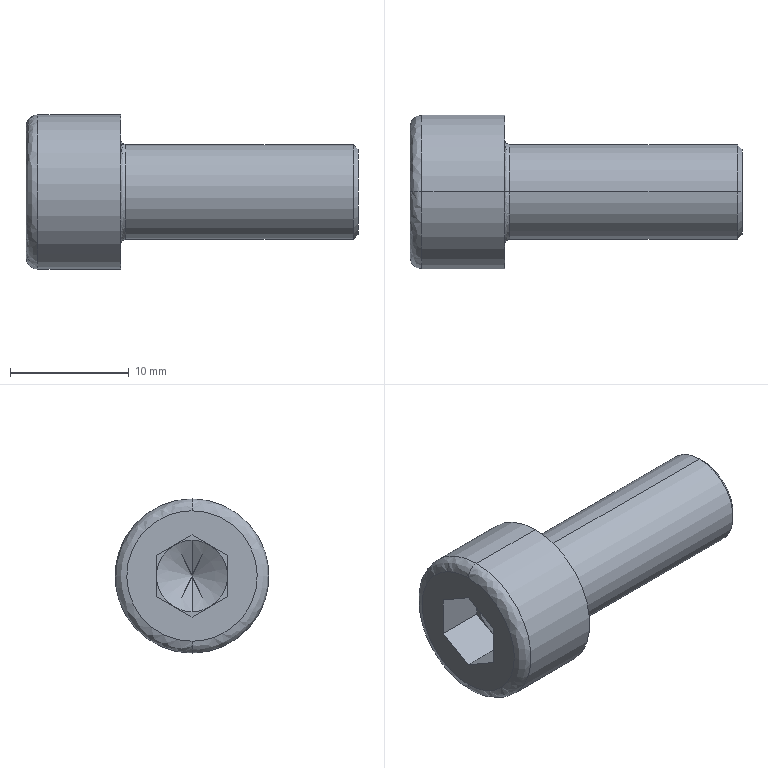Part | SolidWorks | features BaseBody 1 | 1 solid | 27 faces | box 28 x 13 x 13 mm | volume 1917 mm3 | plane 15 | spline 4 | cylinder 4 | cone 4 | commonest cylinder face diameters 8 x2 13 x2
STEP:
#1=CARTESIAN_POINT('',(8.,0.,4.4));
#2=VERTEX_POINT('',#1);
#3=CARTESIAN_POINT('',(8.,0.,-4.4));
#4=VERTEX_POINT('',#3);
#5=CARTESIAN_POINT('',(8.,0.,4.4));
#6=CARTESIAN_POINT('',(8.,0.2797,4.4));
#7=CARTESIAN_POINT('',(8.,0.6919,4.361));
#8=CARTESIAN_POINT('',(8.,1.16,4.249));
#9=CARTESIAN_POINT('',(8.,1.391,4.176));
#10=CARTESIAN_POINT('',(8.,1.489,4.141));
#11=CARTESIAN_POINT('',(8.,1.554,4.116));
#12=CARTESIAN_POINT('',(8.,1.585,4.105));
#13=CARTESIAN_POINT('',(8.,1.758,4.036));
#14=CARTESIAN_POINT('',(8.,1.96,3.944));
#15=CARTESIAN_POINT('',(8.,2.154,3.837));
#16=CARTESIAN_POINT('',(8.,2.282,3.763));
#17=CARTESIAN_POINT('',(8.,2.344,3.724));
#18=CARTESIAN_POINT('',(8.,2.662,3.517));
#19=CARTESIAN_POINT('',(8.,2.897,3.326));
#20=CARTESIAN_POINT('',(8.,3.219,3.004));
#21=CARTESIAN_POINT('',(8.,3.37,2.836));
#22=CARTESIAN_POINT('',(8.,3.509,2.656));
#23=CARTESIAN_POINT('',(8.,3.598,2.534));
#24=CARTESIAN_POINT('',(8.,3.642,2.47));
#25=CARTESIAN_POINT('',(8.,3.764,2.283));
#26=CARTESIAN_POINT('',(8.,3.876,2.092));
#27=CARTESIAN_POINT('',(8.,3.989,1.859));
#28=CARTESIAN_POINT('',(8.,4.042,1.74));
#29=CARTESIAN_POINT('',(8.,4.063,1.689));
#30=CARTESIAN_POINT('',(8.,4.077,1.654));
#31=CARTESIAN_POINT('',(8.,4.085,1.636));
#32=CARTESIAN_POINT('',(8.,4.297,1.1));
#33=CARTESIAN_POINT('',(8.,4.4,0.5592));
#34=CARTESIAN_POINT('',(8.,4.4,-0.2796));
#35=CARTESIAN_POINT('',(8.,4.361,-0.6917));
#36=CARTESIAN_POINT('',(8.,4.249,-1.16));
#37=CARTESIAN_POINT('',(8.,4.176,-1.391));
#38=CARTESIAN_POINT('',(8.,4.141,-1.489));
#39=CARTESIAN_POINT('',(8.,4.116,-1.554));
#40=CARTESIAN_POINT('',(8.,4.105,-1.585));
#41=CARTESIAN_POINT('',(8.,4.036,-1.758));
#42=CARTESIAN_POINT('',(8.,3.944,-1.96));
#43=CARTESIAN_POINT('',(8.,3.837,-2.154));
#44=CARTESIAN_POINT('',(8.,3.763,-2.282));
#45=CARTESIAN_POINT('',(8.,3.724,-2.344));
#46=CARTESIAN_POINT('',(8.,3.517,-2.662));
#47=CARTESIAN_POINT('',(8.,3.326,-2.897));
#48=CARTESIAN_POINT('',(8.,3.004,-3.219));
#49=CARTESIAN_POINT('',(8.,2.836,-3.37));
#50=CARTESIAN_POINT('',(8.,2.656,-3.509));
#51=CARTESIAN_POINT('',(8.,2.534,-3.598));
#52=CARTESIAN_POINT('',(8.,2.47,-3.642));
#53=CARTESIAN_POINT('',(8.,2.283,-3.764));
#54=CARTESIAN_POINT('',(8.,2.092,-3.876));
#55=CARTESIAN_POINT('',(8.,1.859,-3.989));
#56=CARTESIAN_POINT('',(8.,1.74,-4.042));
#57=CARTESIAN_POINT('',(8.,1.689,-4.063));
#58=CARTESIAN_POINT('',(8.,1.654,-4.077));
#59=CARTESIAN_POINT('',(8.,1.636,-4.085));
#60=CARTESIAN_POINT('',(8.,1.1,-4.297));
#61=CARTESIAN_POINT('',(8.,0.5597,-4.4));
#62=CARTESIAN_POINT('',(8.,0.,-4.4));
#63=B_SPLINE_CURVE_WITH_KNOTS('',3,(#5,#6,#7,#8,#9,#10,#11,#12,#13,#14,#15,#16,#17,#18,#19,#20,#21,#22,#23,#24,#25,#26,#27,#28,#29,#30,#31,#32,#33,#34,#35,#36,#37,#38,#39,#40,#41,#42,#43,#44,#45,#46,#47,#48,#49,#50,#51,#52,#53,#54,#55,#56,#57,#58,#59,#60,#61,#62),.UNSPECIFIED.,.F.,.F.,(4,1,1,1,2,2,1,2,2,2,1,2,2,1,1,1,2,2,2,1,1,1,2,2,1,2,2,2,1,2,2,1,1,1,2,2,4),(0.,0.0625,0.09375,0.1094,0.1172,0.125,0.1562,0.1719,0.1875,0.25,0.2812,0.2969,0.3125,0.3437,0.3594,0.3672,0.3711,0.375,0.5,0.5625,0.5937,0.6094,0.6172,0.625,0.6562,0.6719,0.6875,0.75,0.7812,0.7969,0.8125,0.8437,0.8594,0.8672,0.8711,0.875,1.),.UNSPECIFIED.);
#64=EDGE_CURVE('',#2,#4,#63,.T.);
#65=ORIENTED_EDGE('',*,*,#64,.F.);
#66=CARTESIAN_POINT('',(8.4,0.,4.));
#67=VERTEX_POINT('',#66);
#68=CARTESIAN_POINT('',(8.4,0.,4.4));
#69=DIRECTION('',(0.,-1.,0.));
#70=DIRECTION('',(0.,0.,1.));
#71=AXIS2_PLACEMENT_3D('',#68,#69,#70);
#72=CIRCLE('',#71,0.4);
#73=EDGE_CURVE('',#2,#67,#72,.T.);
#74=ORIENTED_EDGE('',*,*,#73,.T.);
#75=CARTESIAN_POINT('',(8.4,0.,-4.));
#76=VERTEX_POINT('',#75);
#77=CARTESIAN_POINT('',(8.4,0.,0.));
#78=DIRECTION('',(1.,0.,0.));
#79=DIRECTION('',(0.,0.,1.));
#80=AXIS2_PLACEMENT_3D('',#77,#78,#79);
#81=CIRCLE('',#80,4.);
#82=EDGE_CURVE('',#76,#67,#81,.T.);
#83=ORIENTED_EDGE('',*,*,#82,.F.);
#84=CARTESIAN_POINT('',(8.4,0.,-4.4));
#85=DIRECTION('',(0.,1.,0.));
#86=DIRECTION('',(0.,0.,-1.));
#87=AXIS2_PLACEMENT_3D('',#84,#85,#86);
#88=CIRCLE('',#87,0.4);
#89=EDGE_CURVE('',#4,#76,#88,.T.);
#90=ORIENTED_EDGE('',*,*,#89,.F.);
#91=EDGE_LOOP('',(#65,#74,#83,#90));
#92=FACE_OUTER_BOUND('',#91,.T.);
#93=CARTESIAN_POINT('',(8.,0.,-4.4));
#94=CARTESIAN_POINT('',(8.,8.8,-4.4));
#95=CARTESIAN_POINT('',(8.,8.8,4.4));
#96=CARTESIAN_POINT('',(8.,0.,4.4));
#97=CARTESIAN_POINT('',(8.,0.,-4.166));
#98=CARTESIAN_POINT('',(8.,8.331,-4.166));
#99=CARTESIAN_POINT('',(8.,8.331,4.166));
#100=CARTESIAN_POINT('',(8.,0.,4.166));
#101=CARTESIAN_POINT('',(8.166,0.,-4.));
#102=CARTESIAN_POINT('',(8.166,8.,-4.));
#103=CARTESIAN_POINT('',(8.166,8.,4.));
#104=CARTESIAN_POINT('',(8.166,0.,4.));
#105=CARTESIAN_POINT('',(8.4,0.,-4.));
#106=CARTESIAN_POINT('',(8.4,8.,-4.));
#107=CARTESIAN_POINT('',(8.4,8.,4.));
#108=CARTESIAN_POINT('',(8.4,0.,4.));
#109=(BOUNDED_SURFACE()B_SPLINE_SURFACE(3,3,((#93,#94,#95,#96),(#97,#98,#99,#100),(#101,#102,#103,#104),(#105,#106,#107,#108)),.UNSPECIFIED.,.F.,.F.,.T.)B_SPLINE_SURFACE_WITH_KNOTS((4,4),(4,4),(0.,1.),(0.,1.),.UNSPECIFIED.)GEOMETRIC_REPRESENTATION_ITEM()RATIONAL_B_SPLINE_SURFACE(((1.,0.3333,0.3333,1.),(0.8047,0.2682,0.2682,0.8047),(0.8047,0.2682,0.2682,0.8047),(1.,0.3333,0.3333,1.)))REPRESENTATION_ITEM('')SURFACE());
#110=ADVANCED_FACE('',(#92),#109,.F.);
#111=CARTESIAN_POINT('',(1.,0.,6.5));
#112=VERTEX_POINT('',#111);
#113=CARTESIAN_POINT('',(1.,0.,-6.5));
#114=VERTEX_POINT('',#113);
#115=CARTESIAN_POINT('',(1.,0.,0.));
#116=DIRECTION('',(1.,0.,0.));
#117=DIRECTION('',(0.,0.,1.));
#118=AXIS2_PLACEMENT_3D('',#115,#116,#117);
#119=CIRCLE('',#118,6.5);
#120=EDGE_CURVE('',#112,#114,#119,.T.);
#121=ORIENTED_EDGE('',*,*,#120,.F.);
#122=CARTESIAN_POINT('',(0.,0.,5.5));
#123=VERTEX_POINT('',#122);
#124=CARTESIAN_POINT('',(1.,0.,5.5));
#125=DIRECTION('',(0.,-1.,0.));
#126=DIRECTION('',(0.,0.,1.));
#127=AXIS2_PLACEMENT_3D('',#124,#125,#126);
#128=CIRCLE('',#127,1.);
#129=EDGE_CURVE('',#112,#123,#128,.T.);
#130=ORIENTED_EDGE('',*,*,#129,.T.);
#131=CARTESIAN_POINT('',(0.,0.,-5.5));
#132=VERTEX_POINT('',#131);
#133=CARTESIAN_POINT('',(0.,0.,5.5));
#134=CARTESIAN_POINT('',(0.,-11.,5.5));
#135=CARTESIAN_POINT('',(0.,-11.,-5.5));
#136=CARTESIAN_POINT('',(0.,0.,-5.5));
#137=(BOUNDED_CURVE()B_SPLINE_CURVE(3,(#133,#134,#135,#136),.UNSPECIFIED.,.F.,.F.)B_SPLINE_CURVE_WITH_KNOTS((4,4),(0.,1.),.UNSPECIFIED.)CURVE()GEOMETRIC_REPRESENTATION_ITEM()RATIONAL_B_SPLINE_CURVE((1.,0.3333,0.3333,1.))REPRESENTATION_ITEM(''));
#138=EDGE_CURVE('',#123,#132,#137,.T.);
#139=ORIENTED_EDGE('',*,*,#138,.T.);
#140=CARTESIAN_POINT('',(1.,0.,-5.5));
#141=DIRECTION('',(0.,1.,0.));
#142=DIRECTION('',(0.,0.,-1.));
#143=AXIS2_PLACEMENT_3D('',#140,#141,#142);
#144=CIRCLE('',#143,1.);
#145=EDGE_CURVE('',#114,#132,#144,.T.);
#146=ORIENTED_EDGE('',*,*,#145,.F.);
#147=EDGE_LOOP('',(#121,#130,#139,#146));
#148=FACE_OUTER_BOUND('',#147,.T.);
#149=CARTESIAN_POINT('',(1.,0.,6.5));
#150=CARTESIAN_POINT('',(1.,-13.,6.5));
#151=CARTESIAN_POINT('',(1.,-13.,-6.5));
#152=CARTESIAN_POINT('',(1.,0.,-6.5));
#153=CARTESIAN_POINT('',(0.4142,0.,6.5));
#154=CARTESIAN_POINT('',(0.4142,-13.,6.5));
#155=CARTESIAN_POINT('',(0.4142,-13.,-6.5));
#156=CARTESIAN_POINT('',(0.4142,0.,-6.5));
#157=CARTESIAN_POINT('',(0.,0.,6.086));
#158=CARTESIAN_POINT('',(0.,-12.172,6.086));
#159=CARTESIAN_POINT('',(0.,-12.172,-6.086));
#160=CARTESIAN_POINT('',(0.,0.,-6.086));
#161=CARTESIAN_POINT('',(0.,0.,5.5));
#162=CARTESIAN_POINT('',(0.,-11.,5.5));
#163=CARTESIAN_POINT('',(0.,-11.,-5.5));
#164=CARTESIAN_POINT('',(0.,0.,-5.5));
#165=(BOUNDED_SURFACE()B_SPLINE_SURFACE(3,3,((#149,#150,#151,#152),(#153,#154,#155,#156),(#157,#158,#159,#160),(#161,#162,#163,#164)),.UNSPECIFIED.,.F.,.F.,.F.)B_SPLINE_SURFACE_WITH_KNOTS((4,4),(4,4),(0.,1.),(0.,1.),.UNSPECIFIED.)GEOMETRIC_REPRESENTATION_ITEM()RATIONAL_B_SPLINE_SURFACE(((1.,0.3333,0.3333,1.),(0.8047,0.2682,0.2682,0.8047),(0.8047,0.2682,0.2682,0.8047),(1.,0.3333,0.3333,1.)))REPRESENTATION_ITEM('')SURFACE());
#166=ADVANCED_FACE('',(#148),#165,.T.);
#167=CARTESIAN_POINT('',(27.6,0.,4.));
#168=VERTEX_POINT('',#167);
#169=CARTESIAN_POINT('',(27.6,0.,-4.));
#170=VERTEX_POINT('',#169);
#171=CARTESIAN_POINT('',(27.6,0.,0.));
#172=DIRECTION('',(-1.,0.,0.));
#173=DIRECTION('',(0.,0.,1.));
#174=AXIS2_PLACEMENT_3D('',#171,#172,#173);
#175=CIRCLE('',#174,4.);
#176=EDGE_CURVE('',#168,#170,#175,.T.);
#177=ORIENTED_EDGE('',*,*,#176,.T.);
#178=CARTESIAN_POINT('',(28.,0.,-4.));
#179=DIRECTION('',(-1.,0.,0.));
#180=VECTOR('',#179,1000.);
#181=LINE('',#178,#180);
#182=EDGE_CURVE('',#170,#76,#181,.T.);
#183=ORIENTED_EDGE('',*,*,#182,.T.);
#184=ORIENTED_EDGE('',*,*,#82,.T.);
#185=CARTESIAN_POINT('',(28.,0.,4.));
#186=DIRECTION('',(-1.,0.,0.));
#187=VECTOR('',#186,1000.);
#188=LINE('',#185,#187);
#189=EDGE_CURVE('',#168,#67,#188,.T.);
#190=ORIENTED_EDGE('',*,*,#189,.F.);
#191=EDGE_LOOP('',(#177,#183,#184,#190));
#192=FACE_OUTER_BOUND('',#191,.T.);
#193=CARTESIAN_POINT('',(28.,0.,0.));
#194=DIRECTION('',(-1.,0.,0.));
#195=DIRECTION('',(0.,0.,1.));
#196=AXIS2_PLACEMENT_3D('',#193,#194,#195);
#197=CYLINDRICAL_SURFACE('',#196,4.);
#198=ADVANCED_FACE('',(#192),#197,.T.);
#199=CARTESIAN_POINT('',(28.,0.,3.6));
#200=VERTEX_POINT('',#199);
#201=CARTESIAN_POINT('',(28.,0.,-3.6));
#202=VERTEX_POINT('',#201);
#203=CARTESIAN_POINT('',(28.,0.,0.));
#204=DIRECTION('',(-1.,0.,0.));
#205=DIRECTION('',(0.,0.,1.));
#206=AXIS2_PLACEMENT_3D('',#203,#204,#205);
#207=CIRCLE('',#206,3.6);
#208=EDGE_CURVE('',#200,#202,#207,.T.);
#209=ORIENTED_EDGE('',*,*,#208,.T.);
#210=CARTESIAN_POINT('',(27.6,0.,-4.));
#211=DIRECTION('',(-0.7071,0.,-0.7071));
#212=VECTOR('',#211,1000.);
#213=LINE('',#210,#212);
#214=EDGE_CURVE('',#202,#170,#213,.T.);
#215=ORIENTED_EDGE('',*,*,#214,.T.);
#216=ORIENTED_EDGE('',*,*,#176,.F.);
#217=CARTESIAN_POINT('',(27.6,0.,4.));
#218=DIRECTION('',(-0.7071,0.,0.7071));
#219=VECTOR('',#218,1000.);
#220=LINE('',#217,#219);
#221=EDGE_CURVE('',#200,#168,#220,.T.);
#222=ORIENTED_EDGE('',*,*,#221,.F.);
#223=EDGE_LOOP('',(#209,#215,#216,#222));
#224=FACE_OUTER_BOUND('',#223,.T.);
#225=CARTESIAN_POINT('',(27.6,0.,0.));
#226=DIRECTION('',(-1.,0.,0.));
#227=DIRECTION('',(0.,0.,1.));
#228=AXIS2_PLACEMENT_3D('',#225,#226,#227);
#229=CONICAL_SURFACE('',#228,4.,0.7854);
#230=ADVANCED_FACE('',(#224),#229,.T.);
#231=CARTESIAN_POINT('',(8.,0.,-6.5));
#232=VERTEX_POINT('',#231);
#233=CARTESIAN_POINT('',(8.,0.,6.5));
#234=VERTEX_POINT('',#233);
#235=CARTESIAN_POINT('',(8.,0.,0.));
#236=DIRECTION('',(1.,0.,0.));
#237=DIRECTION('',(0.,0.,1.));
#238=AXIS2_PLACEMENT_3D('',#235,#236,#237);
#239=CIRCLE('',#238,6.5);
#240=EDGE_CURVE('',#232,#234,#239,.T.);
#241=ORIENTED_EDGE('',*,*,#240,.F.);
#242=CARTESIAN_POINT('',(8.,0.,-6.5));
#243=DIRECTION('',(-1.,0.,0.));
#244=VECTOR('',#243,1000.);
#245=LINE('',#242,#244);
#246=EDGE_CURVE('',#232,#114,#245,.T.);
#247=ORIENTED_EDGE('',*,*,#246,.T.);
#248=CARTESIAN_POINT('',(1.,0.,0.));
#249=DIRECTION('',(1.,0.,0.));
#250=DIRECTION('',(0.,0.,1.));
#251=AXIS2_PLACEMENT_3D('',#248,#249,#250);
#252=CIRCLE('',#251,6.5);
#253=EDGE_CURVE('',#114,#112,#252,.T.);
#254=ORIENTED_EDGE('',*,*,#253,.T.);
#255=CARTESIAN_POINT('',(8.,0.,6.5));
#256=DIRECTION('',(-1.,0.,0.));
#257=VECTOR('',#256,1000.);
#258=LINE('',#255,#257);
#259=EDGE_CURVE('',#234,#112,#258,.T.);
#260=ORIENTED_EDGE('',*,*,#259,.F.);
#261=EDGE_LOOP('',(#241,#247,#254,#260));
#262=FACE_OUTER_BOUND('',#261,.T.);
#263=CARTESIAN_POINT('',(8.,0.,0.));
#264=DIRECTION('',(-1.,0.,0.));
#265=DIRECTION('',(0.,0.,1.));
#266=AXIS2_PLACEMENT_3D('',#263,#264,#265);
#267=CYLINDRICAL_SURFACE('',#266,6.5);
#268=ADVANCED_FACE('',(#262),#267,.T.);
#269=CARTESIAN_POINT('',(5.732,0.,0.));
#270=VERTEX_POINT('',#269);
#271=CARTESIAN_POINT('',(4.,0.,3.));
#272=VERTEX_POINT('',#271);
#273=CARTESIAN_POINT('',(4.,0.,3.));
#274=DIRECTION('',(-0.5,0.,0.866));
#275=VECTOR('',#274,1000.);
#276=LINE('',#273,#275);
#277=EDGE_CURVE('',#270,#272,#276,.T.);
#278=ORIENTED_EDGE('',*,*,#277,.F.);
#279=CARTESIAN_POINT('',(4.,0.,-3.));
#280=VERTEX_POINT('',#279);
#281=CARTESIAN_POINT('',(4.,0.,-3.));
#282=DIRECTION('',(-0.5,0.,-0.866));
#283=VECTOR('',#282,1000.);
#284=LINE('',#281,#283);
#285=EDGE_CURVE('',#270,#280,#284,.T.);
#286=ORIENTED_EDGE('',*,*,#285,.T.);
#287=CARTESIAN_POINT('',(4.,-1.5,-2.598));
#288=VERTEX_POINT('',#287);
#289=CARTESIAN_POINT('',(4.,0.,0.));
#290=DIRECTION('',(1.,0.,0.));
#291=DIRECTION('',(0.,0.,1.));
#292=AXIS2_PLACEMENT_3D('',#289,#290,#291);
#293=CIRCLE('',#292,3.);
#294=EDGE_CURVE('',#288,#280,#293,.T.);
#295=ORIENTED_EDGE('',*,*,#294,.F.);
#296=CARTESIAN_POINT('',(4.,-3.,0.));
#297=VERTEX_POINT('',#296);
#298=CARTESIAN_POINT('',(4.,0.,0.));
#299=DIRECTION('',(-1.,0.,0.));
#300=DIRECTION('',(0.,0.,1.));
#301=AXIS2_PLACEMENT_3D('',#298,#299,#300);
#302=CIRCLE('',#301,3.);
#303=EDGE_CURVE('',#288,#297,#302,.T.);
#304=ORIENTED_EDGE('',*,*,#303,.T.);
#305=CARTESIAN_POINT('',(4.,-1.5,2.598));
#306=VERTEX_POINT('',#305);
#307=CARTESIAN_POINT('',(4.,0.,0.));
#308=DIRECTION('',(1.,0.,0.));
#309=DIRECTION('',(0.,0.,1.));
#310=AXIS2_PLACEMENT_3D('',#307,#308,#309);
#311=CIRCLE('',#310,3.);
#312=EDGE_CURVE('',#306,#297,#311,.T.);
#313=ORIENTED_EDGE('',*,*,#312,.F.);
#314=CARTESIAN_POINT('',(4.,0.,0.));
#315=DIRECTION('',(1.,0.,0.));
#316=DIRECTION('',(0.,0.,1.));
#317=AXIS2_PLACEMENT_3D('',#314,#315,#316);
#318=CIRCLE('',#317,3.);
#319=EDGE_CURVE('',#272,#306,#318,.T.);
#320=ORIENTED_EDGE('',*,*,#319,.F.);
#321=EDGE_LOOP('',(#278,#286,#295,#304,#313,#320));
#322=FACE_OUTER_BOUND('',#321,.T.);
#323=CARTESIAN_POINT('',(4.,0.,0.));
#324=DIRECTION('',(-1.,0.,0.));
#325=DIRECTION('',(0.,0.,1.));
#326=AXIS2_PLACEMENT_3D('',#323,#324,#325);
#327=CONICAL_SURFACE('',#326,3.,1.047);
#328=ADVANCED_FACE('',(#322),#327,.F.);
#329=ORIENTED_EDGE('',*,*,#182,.F.);
#330=CARTESIAN_POINT('',(27.6,0.,0.));
#331=DIRECTION('',(-1.,0.,0.));
#332=DIRECTION('',(0.,0.,1.));
#333=AXIS2_PLACEMENT_3D('',#330,#331,#332);
#334=CIRCLE('',#333,4.);
#335=EDGE_CURVE('',#170,#168,#334,.T.);
#336=ORIENTED_EDGE('',*,*,#335,.T.);
#337=ORIENTED_EDGE('',*,*,#189,.T.);
#338=CARTESIAN_POINT('',(8.4,0.,0.));
#339=DIRECTION('',(1.,0.,0.));
#340=DIRECTION('',(0.,0.,1.));
#341=AXIS2_PLACEMENT_3D('',#338,#339,#340);
#342=CIRCLE('',#341,4.);
#343=EDGE_CURVE('',#67,#76,#342,.T.);
#344=ORIENTED_EDGE('',*,*,#343,.T.);
#345=EDGE_LOOP('',(#329,#336,#337,#344));
#346=FACE_OUTER_BOUND('',#345,.T.);
#347=CARTESIAN_POINT('',(28.,0.,0.));
#348=DIRECTION('',(-1.,0.,0.));
#349=DIRECTION('',(0.,0.,1.));
#350=AXIS2_PLACEMENT_3D('',#347,#348,#349);
#351=CYLINDRICAL_SURFACE('',#350,4.);
#352=ADVANCED_FACE('',(#346),#351,.T.);
#353=ORIENTED_EDGE('',*,*,#73,.F.);
#354=CARTESIAN_POINT('',(8.,0.,-4.4));
#355=CARTESIAN_POINT('',(8.,-0.2797,-4.4));
#356=CARTESIAN_POINT('',(8.,-0.6919,-4.361));
#357=CARTESIAN_POINT('',(8.,-1.16,-4.249));
#358=CARTESIAN_POINT('',(8.,-1.391,-4.176));
#359=CARTESIAN_POINT('',(8.,-1.489,-4.141));
#360=CARTESIAN_POINT('',(8.,-1.554,-4.116));
#361=CARTESIAN_POINT('',(8.,-1.585,-4.105));
#362=CARTESIAN_POINT('',(8.,-1.758,-4.036));
#363=CARTESIAN_POINT('',(8.,-1.96,-3.944));
#364=CARTESIAN_POINT('',(8.,-2.154,-3.837));
#365=CARTESIAN_POINT('',(8.,-2.282,-3.763));
#366=CARTESIAN_POINT('',(8.,-2.344,-3.724));
#367=CARTESIAN_POINT('',(8.,-2.662,-3.517));
#368=CARTESIAN_POINT('',(8.,-2.897,-3.326));
#369=CARTESIAN_POINT('',(8.,-3.219,-3.004));
#370=CARTESIAN_POINT('',(8.,-3.37,-2.836));
#371=CARTESIAN_POINT('',(8.,-3.509,-2.656));
#372=CARTESIAN_POINT('',(8.,-3.598,-2.534));
#373=CARTESIAN_POINT('',(8.,-3.642,-2.47));
#374=CARTESIAN_POINT('',(8.,-3.764,-2.283));
#375=CARTESIAN_POINT('',(8.,-3.876,-2.092));
#376=CARTESIAN_POINT('',(8.,-3.989,-1.859));
#377=CARTESIAN_POINT('',(8.,-4.042,-1.74));
#378=CARTESIAN_POINT('',(8.,-4.063,-1.689));
#379=CARTESIAN_POINT('',(8.,-4.077,-1.654));
#380=CARTESIAN_POINT('',(8.,-4.085,-1.636));
#381=CARTESIAN_POINT('',(8.,-4.297,-1.1));
#382=CARTESIAN_POINT('',(8.,-4.4,-0.5592));
#383=CARTESIAN_POINT('',(8.,-4.4,0.2796));
#384=CARTESIAN_POINT('',(8.,-4.361,0.6917));
#385=CARTESIAN_POINT('',(8.,-4.249,1.16));
#386=CARTESIAN_POINT('',(8.,-4.176,1.391));
#387=CARTESIAN_POINT('',(8.,-4.141,1.489));
#388=CARTESIAN_POINT('',(8.,-4.116,1.554));
#389=CARTESIAN_POINT('',(8.,-4.105,1.585));
#390=CARTESIAN_POINT('',(8.,-4.036,1.758));
#391=CARTESIAN_POINT('',(8.,-3.944,1.96));
#392=CARTESIAN_POINT('',(8.,-3.837,2.154));
#393=CARTESIAN_POINT('',(8.,-3.763,2.282));
#394=CARTESIAN_POINT('',(8.,-3.724,2.344));
#395=CARTESIAN_POINT('',(8.,-3.517,2.662));
#396=CARTESIAN_POINT('',(8.,-3.326,2.897));
#397=CARTESIAN_POINT('',(8.,-3.004,3.219));
#398=CARTESIAN_POINT('',(8.,-2.836,3.37));
#399=CARTESIAN_POINT('',(8.,-2.656,3.509));
#400=CARTESIAN_POINT('',(8.,-2.534,3.598));
#401=CARTESIAN_POINT('',(8.,-2.47,3.642));
#402=CARTESIAN_POINT('',(8.,-2.283,3.764));
#403=CARTESIAN_POINT('',(8.,-2.092,3.876));
#404=CARTESIAN_POINT('',(8.,-1.859,3.989));
#405=CARTESIAN_POINT('',(8.,-1.74,4.042));
#406=CARTESIAN_POINT('',(8.,-1.689,4.063));
#407=CARTESIAN_POINT('',(8.,-1.654,4.077));
#408=CARTESIAN_POINT('',(8.,-1.636,4.085));
#409=CARTESIAN_POINT('',(8.,-1.1,4.297));
#410=CARTESIAN_POINT('',(8.,-0.5597,4.4));
#411=CARTESIAN_POINT('',(8.,0.,4.4));
#412=B_SPLINE_CURVE_WITH_KNOTS('',3,(#354,#355,#356,#357,#358,#359,#360,#361,#362,#363,#364,#365,#366,#367,#368,#369,#370,#371,#372,#373,#374,#375,#376,#377,#378,#379,#380,#381,#382,#383,#384,#385,#386,#387,#388,#389,#390,#391,#392,#393,#394,#395,#396,#397,#398,#399,#400,#401,#402,#403,#404,#405,#406,#407,#408,#409,#410,#411),.UNSPECIFIED.,.F.,.F.,(4,1,1,1,2,2,1,2,2,2,1,2,2,1,1,1,2,2,2,1,1,1,2,2,1,2,2,2,1,2,2,1,1,1,2,2,4),(0.,0.0625,0.09375,0.1094,0.1172,0.125,0.1563,0.1719,0.1875,0.25,0.2813,0.2969,0.3125,0.3438,0.3594,0.3672,0.3711,0.375,0.5,0.5625,0.5938,0.6094,0.6172,0.625,0.6563,0.6719,0.6875,0.75,0.7813,0.7969,0.8125,0.8438,0.8594,0.8672,0.8711,0.875,1.),.UNSPECIFIED.);
#413=EDGE_CURVE('',#4,#2,#412,.T.);
#414=ORIENTED_EDGE('',*,*,#413,.F.);
#415=ORIENTED_EDGE('',*,*,#89,.T.);
#416=ORIENTED_EDGE('',*,*,#343,.F.);
#417=EDGE_LOOP('',(#353,#414,#415,#416));
#418=FACE_OUTER_BOUND('',#417,.T.);
#419=CARTESIAN_POINT('',(8.,0.,4.4));
#420=CARTESIAN_POINT('',(8.,-8.8,4.4));
#421=CARTESIAN_POINT('',(8.,-8.8,-4.4));
#422=CARTESIAN_POINT('',(8.,0.,-4.4));
#423=CARTESIAN_POINT('',(8.,0.,4.166));
#424=CARTESIAN_POINT('',(8.,-8.331,4.166));
#425=CARTESIAN_POINT('',(8.,-8.331,-4.166));
#426=CARTESIAN_POINT('',(8.,0.,-4.166));
#427=CARTESIAN_POINT('',(8.166,0.,4.));
#428=CARTESIAN_POINT('',(8.166,-8.,4.));
#429=CARTESIAN_POINT('',(8.166,-8.,-4.));
#430=CARTESIAN_POINT('',(8.166,0.,-4.));
#431=CARTESIAN_POINT('',(8.4,0.,4.));
#432=CARTESIAN_POINT('',(8.4,-8.,4.));
#433=CARTESIAN_POINT('',(8.4,-8.,-4.));
#434=CARTESIAN_POINT('',(8.4,0.,-4.));
#435=(BOUNDED_SURFACE()B_SPLINE_SURFACE(3,3,((#419,#420,#421,#422),(#423,#424,#425,#426),(#427,#428,#429,#430),(#431,#432,#433,#434)),.UNSPECIFIED.,.F.,.F.,.T.)B_SPLINE_SURFACE_WITH_KNOTS((4,4),(4,4),(0.,1.),(0.,1.),.UNSPECIFIED.)GEOMETRIC_REPRESENTATION_ITEM()RATIONAL_B_SPLINE_SURFACE(((1.,0.3333,0.3333,1.),(0.8047,0.2682,0.2682,0.8047),(0.8047,0.2682,0.2682,0.8047),(1.,0.3333,0.3333,1.)))REPRESENTATION_ITEM('')SURFACE());
#436=ADVANCED_FACE('',(#418),#435,.F.);
#437=ORIENTED_EDGE('',*,*,#214,.F.);
#438=CARTESIAN_POINT('',(28.,0.,0.));
#439=DIRECTION('',(-1.,0.,0.));
#440=DIRECTION('',(0.,0.,1.));
#441=AXIS2_PLACEMENT_3D('',#438,#439,#440);
#442=CIRCLE('',#441,3.6);
#443=EDGE_CURVE('',#202,#200,#442,.T.);
#444=ORIENTED_EDGE('',*,*,#443,.T.);
#445=ORIENTED_EDGE('',*,*,#221,.T.);
#446=ORIENTED_EDGE('',*,*,#335,.F.);
#447=EDGE_LOOP('',(#437,#444,#445,#446));
#448=FACE_OUTER_BOUND('',#447,.T.);
#449=CARTESIAN_POINT('',(27.6,0.,0.));
#450=DIRECTION('',(-1.,0.,0.));
#451=DIRECTION('',(0.,0.,1.));
#452=AXIS2_PLACEMENT_3D('',#449,#450,#451);
#453=CONICAL_SURFACE('',#452,4.,0.7854);
#454=ADVANCED_FACE('',(#448),#453,.T.);
#455=CARTESIAN_POINT('',(8.,0.,0.));
#456=DIRECTION('',(1.,0.,0.));
#457=DIRECTION('',(0.,0.,1.));
#458=AXIS2_PLACEMENT_3D('',#455,#456,#457);
#459=CIRCLE('',#458,6.5);
#460=EDGE_CURVE('',#234,#232,#459,.T.);
#461=ORIENTED_EDGE('',*,*,#460,.T.);
#462=ORIENTED_EDGE('',*,*,#240,.T.);
#463=EDGE_LOOP('',(#461,#462));
#464=FACE_OUTER_BOUND('',#463,.T.);
#465=ORIENTED_EDGE('',*,*,#413,.T.);
#466=ORIENTED_EDGE('',*,*,#64,.T.);
#467=EDGE_LOOP('',(#465,#466));
#468=FACE_BOUND('',#467,.T.);
#469=CARTESIAN_POINT('',(8.,0.,0.));
#470=DIRECTION('',(1.,0.,0.));
#471=DIRECTION('',(0.,0.,-1.));
#472=AXIS2_PLACEMENT_3D('',#469,#470,#471);
#473=PLANE('',#472);
#474=ADVANCED_FACE('',(#464,#468),#473,.T.);
#475=ORIENTED_EDGE('',*,*,#208,.F.);
#476=ORIENTED_EDGE('',*,*,#443,.F.);
#477=EDGE_LOOP('',(#475,#476));
#478=FACE_OUTER_BOUND('',#477,.T.);
#479=CARTESIAN_POINT('',(28.,0.,0.));
#480=DIRECTION('',(1.,0.,0.));
#481=DIRECTION('',(0.,0.,-1.));
#482=AXIS2_PLACEMENT_3D('',#479,#480,#481);
#483=PLANE('',#482);
#484=ADVANCED_FACE('',(#478),#483,.T.);
#485=ORIENTED_EDGE('',*,*,#246,.F.);
#486=ORIENTED_EDGE('',*,*,#460,.F.);
#487=ORIENTED_EDGE('',*,*,#259,.T.);
#488=ORIENTED_EDGE('',*,*,#120,.T.);
#489=EDGE_LOOP('',(#485,#486,#487,#488));
#490=FACE_OUTER_BOUND('',#489,.T.);
#491=CARTESIAN_POINT('',(8.,0.,0.));
#492=DIRECTION('',(-1.,0.,0.));
#493=DIRECTION('',(0.,0.,1.));
#494=AXIS2_PLACEMENT_3D('',#491,#492,#493);
#495=CYLINDRICAL_SURFACE('',#494,6.5);
#496=ADVANCED_FACE('',(#490),#495,.T.);
#497=ORIENTED_EDGE('',*,*,#129,.F.);
#498=ORIENTED_EDGE('',*,*,#253,.F.);
#499=ORIENTED_EDGE('',*,*,#145,.T.);
#500=CARTESIAN_POINT('',(0.,0.,-5.5));
#501=CARTESIAN_POINT('',(0.,11.,-5.5));
#502=CARTESIAN_POINT('',(0.,11.,5.5));
#503=CARTESIAN_POINT('',(0.,0.,5.5));
#504=(BOUNDED_CURVE()B_SPLINE_CURVE(3,(#500,#501,#502,#503),.UNSPECIFIED.,.F.,.F.)B_SPLINE_CURVE_WITH_KNOTS((4,4),(0.,1.),.UNSPECIFIED.)CURVE()GEOMETRIC_REPRESENTATION_ITEM()RATIONAL_B_SPLINE_CURVE((1.,0.3333,0.3333,1.))REPRESENTATION_ITEM(''));
#505=EDGE_CURVE('',#132,#123,#504,.T.);
#506=ORIENTED_EDGE('',*,*,#505,.T.);
#507=EDGE_LOOP('',(#497,#498,#499,#506));
#508=FACE_OUTER_BOUND('',#507,.T.);
#509=CARTESIAN_POINT('',(1.,0.,-6.5));
#510=CARTESIAN_POINT('',(1.,13.,-6.5));
#511=CARTESIAN_POINT('',(1.,13.,6.5));
#512=CARTESIAN_POINT('',(1.,0.,6.5));
#513=CARTESIAN_POINT('',(0.4142,0.,-6.5));
#514=CARTESIAN_POINT('',(0.4142,13.,-6.5));
#515=CARTESIAN_POINT('',(0.4142,13.,6.5));
#516=CARTESIAN_POINT('',(0.4142,0.,6.5));
#517=CARTESIAN_POINT('',(0.,0.,-6.086));
#518=CARTESIAN_POINT('',(0.,12.172,-6.086));
#519=CARTESIAN_POINT('',(0.,12.172,6.086));
#520=CARTESIAN_POINT('',(0.,0.,6.086));
#521=CARTESIAN_POINT('',(0.,0.,-5.5));
#522=CARTESIAN_POINT('',(0.,11.,-5.5));
#523=CARTESIAN_POINT('',(0.,11.,5.5));
#524=CARTESIAN_POINT('',(0.,0.,5.5));
#525=(BOUNDED_SURFACE()B_SPLINE_SURFACE(3,3,((#509,#510,#511,#512),(#513,#514,#515,#516),(#517,#518,#519,#520),(#521,#522,#523,#524)),.UNSPECIFIED.,.F.,.F.,.F.)B_SPLINE_SURFACE_WITH_KNOTS((4,4),(4,4),(0.,1.),(0.,1.),.UNSPECIFIED.)GEOMETRIC_REPRESENTATION_ITEM()RATIONAL_B_SPLINE_SURFACE(((1.,0.3333,0.3333,1.),(0.8047,0.2682,0.2682,0.8047),(0.8047,0.2682,0.2682,0.8047),(1.,0.3333,0.3333,1.)))REPRESENTATION_ITEM('')SURFACE());
#526=ADVANCED_FACE('',(#508),#525,.T.);
#527=CARTESIAN_POINT('',(0.,3.,1.732));
#528=VERTEX_POINT('',#527);
#529=CARTESIAN_POINT('',(0.,3.,-1.732));
#530=VERTEX_POINT('',#529);
#531=CARTESIAN_POINT('',(0.,3.,0.));
#532=DIRECTION('',(0.,0.,-1.));
#533=VECTOR('',#532,1000.);
#534=LINE('',#531,#533);
#535=EDGE_CURVE('',#528,#530,#534,.T.);
#536=ORIENTED_EDGE('',*,*,#535,.F.);
#537=CARTESIAN_POINT('',(0.,0.,3.464));
#538=VERTEX_POINT('',#537);
#539=CARTESIAN_POINT('',(0.,0.,3.464));
#540=DIRECTION('',(0.,0.866,-0.5));
#541=VECTOR('',#540,1000.);
#542=LINE('',#539,#541);
#543=EDGE_CURVE('',#538,#528,#542,.T.);
#544=ORIENTED_EDGE('',*,*,#543,.F.);
#545=CARTESIAN_POINT('',(0.,-3.,1.732));
#546=VERTEX_POINT('',#545);
#547=CARTESIAN_POINT('',(0.,-3.,1.732));
#548=DIRECTION('',(0.,0.866,0.5));
#549=VECTOR('',#548,1000.);
#550=LINE('',#547,#549);
#551=EDGE_CURVE('',#546,#538,#550,.T.);
#552=ORIENTED_EDGE('',*,*,#551,.F.);
#553=CARTESIAN_POINT('',(0.,-3.,-1.732));
#554=VERTEX_POINT('',#553);
#555=CARTESIAN_POINT('',(0.,-3.,0.));
#556=DIRECTION('',(0.,0.,1.));
#557=VECTOR('',#556,1000.);
#558=LINE('',#555,#557);
#559=EDGE_CURVE('',#554,#546,#558,.T.);
#560=ORIENTED_EDGE('',*,*,#559,.F.);
#561=CARTESIAN_POINT('',(0.,0.,-3.464));
#562=VERTEX_POINT('',#561);
#563=CARTESIAN_POINT('',(0.,0.,-3.464));
#564=DIRECTION('',(0.,-0.866,0.5));
#565=VECTOR('',#564,1000.);
#566=LINE('',#563,#565);
#567=EDGE_CURVE('',#562,#554,#566,.T.);
#568=ORIENTED_EDGE('',*,*,#567,.F.);
#569=CARTESIAN_POINT('',(0.,3.,-1.732));
#570=DIRECTION('',(0.,-0.866,-0.5));
#571=VECTOR('',#570,1000.);
#572=LINE('',#569,#571);
#573=EDGE_CURVE('',#530,#562,#572,.T.);
#574=ORIENTED_EDGE('',*,*,#573,.F.);
#575=EDGE_LOOP('',(#536,#544,#552,#560,#568,#574));
#576=FACE_BOUND('',#575,.T.);
#577=ORIENTED_EDGE('',*,*,#505,.F.);
#578=ORIENTED_EDGE('',*,*,#138,.F.);
#579=EDGE_LOOP('',(#577,#578));
#580=FACE_OUTER_BOUND('',#579,.T.);
#581=CARTESIAN_POINT('',(0.,0.,0.));
#582=DIRECTION('',(1.,0.,0.));
#583=DIRECTION('',(0.,0.,-1.));
#584=AXIS2_PLACEMENT_3D('',#581,#582,#583);
#585=PLANE('',#584);
#586=ADVANCED_FACE('',(#576,#580),#585,.F.);
#587=CARTESIAN_POINT('',(4.,0.,-3.464));
#588=VERTEX_POINT('',#587);
#589=CARTESIAN_POINT('',(4.,0.,-3.464));
#590=DIRECTION('',(1.,0.,0.));
#591=VECTOR('',#590,1000.);
#592=LINE('',#589,#591);
#593=EDGE_CURVE('',#562,#588,#592,.T.);
#594=ORIENTED_EDGE('',*,*,#593,.T.);
#595=CARTESIAN_POINT('',(4.,1.5,-2.598));
#596=VERTEX_POINT('',#595);
#597=CARTESIAN_POINT('',(4.,0.,-3.464));
#598=DIRECTION('',(0.,0.866,0.5));
#599=VECTOR('',#598,1000.);
#600=LINE('',#597,#599);
#601=EDGE_CURVE('',#588,#596,#600,.T.);
#602=ORIENTED_EDGE('',*,*,#601,.T.);
#603=CARTESIAN_POINT('',(4.,3.,-1.732));
#604=VERTEX_POINT('',#603);
#605=CARTESIAN_POINT('',(4.,1.5,-2.598));
#606=DIRECTION('',(0.,0.866,0.5));
#607=VECTOR('',#606,1000.);
#608=LINE('',#605,#607);
#609=EDGE_CURVE('',#596,#604,#608,.T.);
#610=ORIENTED_EDGE('',*,*,#609,.T.);
#611=CARTESIAN_POINT('',(4.,3.,-1.732));
#612=DIRECTION('',(-1.,0.,0.));
#613=VECTOR('',#612,1000.);
#614=LINE('',#611,#613);
#615=EDGE_CURVE('',#604,#530,#614,.T.);
#616=ORIENTED_EDGE('',*,*,#615,.T.);
#617=ORIENTED_EDGE('',*,*,#573,.T.);
#618=EDGE_LOOP('',(#594,#602,#610,#616,#617));
#619=FACE_OUTER_BOUND('',#618,.T.);
#620=CARTESIAN_POINT('',(4.,0.,-3.464));
#621=DIRECTION('',(0.,-0.5,0.866));
#622=DIRECTION('',(0.,-0.866,-0.5));
#623=AXIS2_PLACEMENT_3D('',#620,#621,#622);
#624=PLANE('',#623);
#625=ADVANCED_FACE('',(#619),#624,.T.);
#626=ORIENTED_EDGE('',*,*,#615,.F.);
#627=CARTESIAN_POINT('',(4.,3.,0.));
#628=VERTEX_POINT('',#627);
#629=CARTESIAN_POINT('',(4.,3.,-3.464));
#630=DIRECTION('',(0.,0.,1.));
#631=VECTOR('',#630,1000.);
#632=LINE('',#629,#631);
#633=EDGE_CURVE('',#604,#628,#632,.T.);
#634=ORIENTED_EDGE('',*,*,#633,.T.);
#635=CARTESIAN_POINT('',(4.,3.,1.732));
#636=VERTEX_POINT('',#635);
#637=CARTESIAN_POINT('',(4.,3.,-3.464));
#638=DIRECTION('',(0.,0.,1.));
#639=VECTOR('',#638,1000.);
#640=LINE('',#637,#639);
#641=EDGE_CURVE('',#628,#636,#640,.T.);
#642=ORIENTED_EDGE('',*,*,#641,.T.);
#643=CARTESIAN_POINT('',(4.,3.,1.732));
#644=DIRECTION('',(-1.,0.,0.));
#645=VECTOR('',#644,1000.);
#646=LINE('',#643,#645);
#647=EDGE_CURVE('',#636,#528,#646,.T.);
#648=ORIENTED_EDGE('',*,*,#647,.T.);
#649=ORIENTED_EDGE('',*,*,#535,.T.);
#650=EDGE_LOOP('',(#626,#634,#642,#648,#649));
#651=FACE_OUTER_BOUND('',#650,.T.);
#652=CARTESIAN_POINT('',(4.,3.,-1.732));
#653=DIRECTION('',(0.,-1.,0.));
#654=DIRECTION('',(0.,0.,-1.));
#655=AXIS2_PLACEMENT_3D('',#652,#653,#654);
#656=PLANE('',#655);
#657=ADVANCED_FACE('',(#651),#656,.T.);
#658=ORIENTED_EDGE('',*,*,#647,.F.);
#659=CARTESIAN_POINT('',(4.,1.5,2.598));
#660=VERTEX_POINT('',#659);
#661=CARTESIAN_POINT('',(4.,3.,1.732));
#662=DIRECTION('',(0.,-0.866,0.5));
#663=VECTOR('',#662,1000.);
#664=LINE('',#661,#663);
#665=EDGE_CURVE('',#636,#660,#664,.T.);
#666=ORIENTED_EDGE('',*,*,#665,.T.);
#667=CARTESIAN_POINT('',(4.,0.,3.464));
#668=VERTEX_POINT('',#667);
#669=CARTESIAN_POINT('',(4.,3.,1.732));
#670=DIRECTION('',(0.,-0.866,0.5));
#671=VECTOR('',#670,1000.);
#672=LINE('',#669,#671);
#673=EDGE_CURVE('',#660,#668,#672,.T.);
#674=ORIENTED_EDGE('',*,*,#673,.T.);
#675=CARTESIAN_POINT('',(4.,0.,3.464));
#676=DIRECTION('',(-1.,0.,0.));
#677=VECTOR('',#676,1000.);
#678=LINE('',#675,#677);
#679=EDGE_CURVE('',#668,#538,#678,.T.);
#680=ORIENTED_EDGE('',*,*,#679,.T.);
#681=ORIENTED_EDGE('',*,*,#543,.T.);
#682=EDGE_LOOP('',(#658,#666,#674,#680,#681));
#683=FACE_OUTER_BOUND('',#682,.T.);
#684=CARTESIAN_POINT('',(4.,3.,1.732));
#685=DIRECTION('',(0.,-0.5,-0.866));
#686=DIRECTION('',(0.,0.866,-0.5));
#687=AXIS2_PLACEMENT_3D('',#684,#685,#686);
#688=PLANE('',#687);
#689=ADVANCED_FACE('',(#683),#688,.T.);
#690=ORIENTED_EDGE('',*,*,#679,.F.);
#691=CARTESIAN_POINT('',(4.,0.,3.464));
#692=DIRECTION('',(0.,-0.866,-0.5));
#693=VECTOR('',#692,1000.);
#694=LINE('',#691,#693);
#695=EDGE_CURVE('',#668,#306,#694,.T.);
#696=ORIENTED_EDGE('',*,*,#695,.T.);
#697=CARTESIAN_POINT('',(4.,-3.,1.732));
#698=VERTEX_POINT('',#697);
#699=CARTESIAN_POINT('',(4.,-1.5,2.598));
#700=DIRECTION('',(0.,-0.866,-0.5));
#701=VECTOR('',#700,1000.);
#702=LINE('',#699,#701);
#703=EDGE_CURVE('',#306,#698,#702,.T.);
#704=ORIENTED_EDGE('',*,*,#703,.T.);
#705=CARTESIAN_POINT('',(4.,-3.,1.732));
#706=DIRECTION('',(-1.,0.,0.));
#707=VECTOR('',#706,1000.);
#708=LINE('',#705,#707);
#709=EDGE_CURVE('',#698,#546,#708,.T.);
#710=ORIENTED_EDGE('',*,*,#709,.T.);
#711=ORIENTED_EDGE('',*,*,#551,.T.);
#712=EDGE_LOOP('',(#690,#696,#704,#710,#711));
#713=FACE_OUTER_BOUND('',#712,.T.);
#714=CARTESIAN_POINT('',(4.,0.,3.464));
#715=DIRECTION('',(0.,0.5,-0.866));
#716=DIRECTION('',(0.,0.866,0.5));
#717=AXIS2_PLACEMENT_3D('',#714,#715,#716);
#718=PLANE('',#717);
#719=ADVANCED_FACE('',(#713),#718,.T.);
#720=ORIENTED_EDGE('',*,*,#709,.F.);
#721=CARTESIAN_POINT('',(4.,-3.,-3.464));
#722=DIRECTION('',(0.,0.,-1.));
#723=VECTOR('',#722,1000.);
#724=LINE('',#721,#723);
#725=EDGE_CURVE('',#698,#297,#724,.T.);
#726=ORIENTED_EDGE('',*,*,#725,.T.);
#727=CARTESIAN_POINT('',(4.,-3.,-1.732));
#728=VERTEX_POINT('',#727);
#729=CARTESIAN_POINT('',(4.,-3.,1.732));
#730=DIRECTION('',(0.,0.,-1.));
#731=VECTOR('',#730,1000.);
#732=LINE('',#729,#731);
#733=EDGE_CURVE('',#297,#728,#732,.T.);
#734=ORIENTED_EDGE('',*,*,#733,.T.);
#735=CARTESIAN_POINT('',(4.,-3.,-1.732));
#736=DIRECTION('',(-1.,0.,0.));
#737=VECTOR('',#736,1000.);
#738=LINE('',#735,#737);
#739=EDGE_CURVE('',#728,#554,#738,.T.);
#740=ORIENTED_EDGE('',*,*,#739,.T.);
#741=ORIENTED_EDGE('',*,*,#559,.T.);
#742=EDGE_LOOP('',(#720,#726,#734,#740,#741));
#743=FACE_OUTER_BOUND('',#742,.T.);
#744=CARTESIAN_POINT('',(4.,-3.,1.732));
#745=DIRECTION('',(0.,1.,0.));
#746=DIRECTION('',(0.,0.,1.));
#747=AXIS2_PLACEMENT_3D('',#744,#745,#746);
#748=PLANE('',#747);
#749=ADVANCED_FACE('',(#743),#748,.T.);
#750=ORIENTED_EDGE('',*,*,#739,.F.);
#751=CARTESIAN_POINT('',(4.,-3.,-1.732));
#752=DIRECTION('',(0.,0.866,-0.5));
#753=VECTOR('',#752,1000.);
#754=LINE('',#751,#753);
#755=EDGE_CURVE('',#728,#288,#754,.T.);
#756=ORIENTED_EDGE('',*,*,#755,.T.);
#757=CARTESIAN_POINT('',(4.,-3.,-1.732));
#758=DIRECTION('',(0.,0.866,-0.5));
#759=VECTOR('',#758,1000.);
#760=LINE('',#757,#759);
#761=EDGE_CURVE('',#288,#588,#760,.T.);
#762=ORIENTED_EDGE('',*,*,#761,.T.);
#763=ORIENTED_EDGE('',*,*,#593,.F.);
#764=ORIENTED_EDGE('',*,*,#567,.T.);
#765=EDGE_LOOP('',(#750,#756,#762,#763,#764));
#766=FACE_OUTER_BOUND('',#765,.T.);
#767=CARTESIAN_POINT('',(4.,-3.,-1.732));
#768=DIRECTION('',(0.,0.5,0.866));
#769=DIRECTION('',(0.,-0.866,0.5));
#770=AXIS2_PLACEMENT_3D('',#767,#768,#769);
#771=PLANE('',#770);
#772=ADVANCED_FACE('',(#766),#771,.T.);
#773=ORIENTED_EDGE('',*,*,#294,.T.);
#774=CARTESIAN_POINT('',(4.,0.,0.));
#775=DIRECTION('',(1.,0.,0.));
#776=DIRECTION('',(0.,0.,1.));
#777=AXIS2_PLACEMENT_3D('',#774,#775,#776);
#778=CIRCLE('',#777,3.);
#779=EDGE_CURVE('',#280,#596,#778,.T.);
#780=ORIENTED_EDGE('',*,*,#779,.T.);
#781=ORIENTED_EDGE('',*,*,#601,.F.);
#782=ORIENTED_EDGE('',*,*,#761,.F.);
#783=EDGE_LOOP('',(#773,#780,#781,#782));
#784=FACE_OUTER_BOUND('',#783,.T.);
#785=CARTESIAN_POINT('',(4.,0.,-3.464));
#786=DIRECTION('',(1.,0.,0.));
#787=DIRECTION('',(0.,0.,-1.));
#788=AXIS2_PLACEMENT_3D('',#785,#786,#787);
#789=PLANE('',#788);
#790=ADVANCED_FACE('',(#784),#789,.F.);
#791=ORIENTED_EDGE('',*,*,#673,.F.);
#792=CARTESIAN_POINT('',(4.,0.,0.));
#793=DIRECTION('',(1.,0.,0.));
#794=DIRECTION('',(0.,0.,1.));
#795=AXIS2_PLACEMENT_3D('',#792,#793,#794);
#796=CIRCLE('',#795,3.);
#797=EDGE_CURVE('',#660,#272,#796,.T.);
#798=ORIENTED_EDGE('',*,*,#797,.T.);
#799=ORIENTED_EDGE('',*,*,#319,.T.);
#800=ORIENTED_EDGE('',*,*,#695,.F.);
#801=EDGE_LOOP('',(#791,#798,#799,#800));
#802=FACE_OUTER_BOUND('',#801,.T.);
#803=CARTESIAN_POINT('',(4.,0.,-3.464));
#804=DIRECTION('',(1.,0.,0.));
#805=DIRECTION('',(0.,0.,-1.));
#806=AXIS2_PLACEMENT_3D('',#803,#804,#805);
#807=PLANE('',#806);
#808=ADVANCED_FACE('',(#802),#807,.F.);
#809=ORIENTED_EDGE('',*,*,#755,.F.);
#810=ORIENTED_EDGE('',*,*,#733,.F.);
#811=ORIENTED_EDGE('',*,*,#303,.F.);
#812=EDGE_LOOP('',(#809,#810,#811));
#813=FACE_OUTER_BOUND('',#812,.T.);
#814=CARTESIAN_POINT('',(4.,0.,-3.464));
#815=DIRECTION('',(1.,0.,0.));
#816=DIRECTION('',(0.,0.,-1.));
#817=AXIS2_PLACEMENT_3D('',#814,#815,#816);
#818=PLANE('',#817);
#819=ADVANCED_FACE('',(#813),#818,.F.);
#820=ORIENTED_EDGE('',*,*,#285,.F.);
#821=ORIENTED_EDGE('',*,*,#277,.T.);
#822=ORIENTED_EDGE('',*,*,#797,.F.);
#823=CARTESIAN_POINT('',(4.,0.,0.));
#824=DIRECTION('',(1.,0.,0.));
#825=DIRECTION('',(0.,0.,1.));
#826=AXIS2_PLACEMENT_3D('',#823,#824,#825);
#827=CIRCLE('',#826,3.);
#828=EDGE_CURVE('',#628,#660,#827,.T.);
#829=ORIENTED_EDGE('',*,*,#828,.F.);
#830=CARTESIAN_POINT('',(4.,0.,0.));
#831=DIRECTION('',(1.,0.,0.));
#832=DIRECTION('',(0.,0.,1.));
#833=AXIS2_PLACEMENT_3D('',#830,#831,#832);
#834=CIRCLE('',#833,3.);
#835=EDGE_CURVE('',#596,#628,#834,.T.);
#836=ORIENTED_EDGE('',*,*,#835,.F.);
#837=ORIENTED_EDGE('',*,*,#779,.F.);
#838=EDGE_LOOP('',(#820,#821,#822,#829,#836,#837));
#839=FACE_OUTER_BOUND('',#838,.T.);
#840=CARTESIAN_POINT('',(4.,0.,0.));
#841=DIRECTION('',(-1.,0.,0.));
#842=DIRECTION('',(0.,0.,1.));
#843=AXIS2_PLACEMENT_3D('',#840,#841,#842);
#844=CONICAL_SURFACE('',#843,3.,1.047);
#845=ADVANCED_FACE('',(#839),#844,.F.);
#846=ORIENTED_EDGE('',*,*,#725,.F.);
#847=ORIENTED_EDGE('',*,*,#703,.F.);
#848=ORIENTED_EDGE('',*,*,#312,.T.);
#849=EDGE_LOOP('',(#846,#847,#848));
#850=FACE_OUTER_BOUND('',#849,.T.);
#851=CARTESIAN_POINT('',(4.,0.,-3.464));
#852=DIRECTION('',(1.,0.,0.));
#853=DIRECTION('',(0.,0.,-1.));
#854=AXIS2_PLACEMENT_3D('',#851,#852,#853);
#855=PLANE('',#854);
#856=ADVANCED_FACE('',(#850),#855,.F.);
#857=ORIENTED_EDGE('',*,*,#665,.F.);
#858=ORIENTED_EDGE('',*,*,#641,.F.);
#859=ORIENTED_EDGE('',*,*,#828,.T.);
#860=EDGE_LOOP('',(#857,#858,#859));
#861=FACE_OUTER_BOUND('',#860,.T.);
#862=CARTESIAN_POINT('',(4.,0.,-3.464));
#863=DIRECTION('',(1.,0.,0.));
#864=DIRECTION('',(0.,0.,-1.));
#865=AXIS2_PLACEMENT_3D('',#862,#863,#864);
#866=PLANE('',#865);
#867=ADVANCED_FACE('',(#861),#866,.F.);
#868=ORIENTED_EDGE('',*,*,#633,.F.);
#869=ORIENTED_EDGE('',*,*,#609,.F.);
#870=ORIENTED_EDGE('',*,*,#835,.T.);
#871=EDGE_LOOP('',(#868,#869,#870));
#872=FACE_OUTER_BOUND('',#871,.T.);
#873=CARTESIAN_POINT('',(4.,0.,-3.464));
#874=DIRECTION('',(1.,0.,0.));
#875=DIRECTION('',(0.,0.,-1.));
#876=AXIS2_PLACEMENT_3D('',#873,#874,#875);
#877=PLANE('',#876);
#878=ADVANCED_FACE('',(#872),#877,.F.);
#879=CLOSED_SHELL('',(#110,#166,#198,#230,#268,#328,#352,#436,#454,#474,#484,#496,#526,#586,#625,#657,#689,#719,#749,#772,#790,#808,#819,#845,#856,#867,#878));
#880=MANIFOLD_SOLID_BREP('',#879);
#881=CARTESIAN_POINT('',(0.,0.,0.));
#882=DIRECTION('',(0.,0.,1.));
#883=DIRECTION('',(1.,0.,0.));
#884=AXIS2_PLACEMENT_3D('',#881,#882,#883);
#885=(LENGTH_UNIT()NAMED_UNIT(*)SI_UNIT(.MILLI.,.METRE.));
#886=UNCERTAINTY_MEASURE_WITH_UNIT(LENGTH_MEASURE(0.00001),#885,'','');
#887=(NAMED_UNIT(*)PLANE_ANGLE_UNIT()SI_UNIT($,.RADIAN.));
#888=(NAMED_UNIT(*)SI_UNIT($,.STERADIAN.)SOLID_ANGLE_UNIT());
#889=(GEOMETRIC_REPRESENTATION_CONTEXT(3)GLOBAL_UNCERTAINTY_ASSIGNED_CONTEXT((#886))GLOBAL_UNIT_ASSIGNED_CONTEXT((#885,#887,#888))REPRESENTATION_CONTEXT('',''));
#890=ADVANCED_BREP_SHAPE_REPRESENTATION('',(#880,#884),#889);